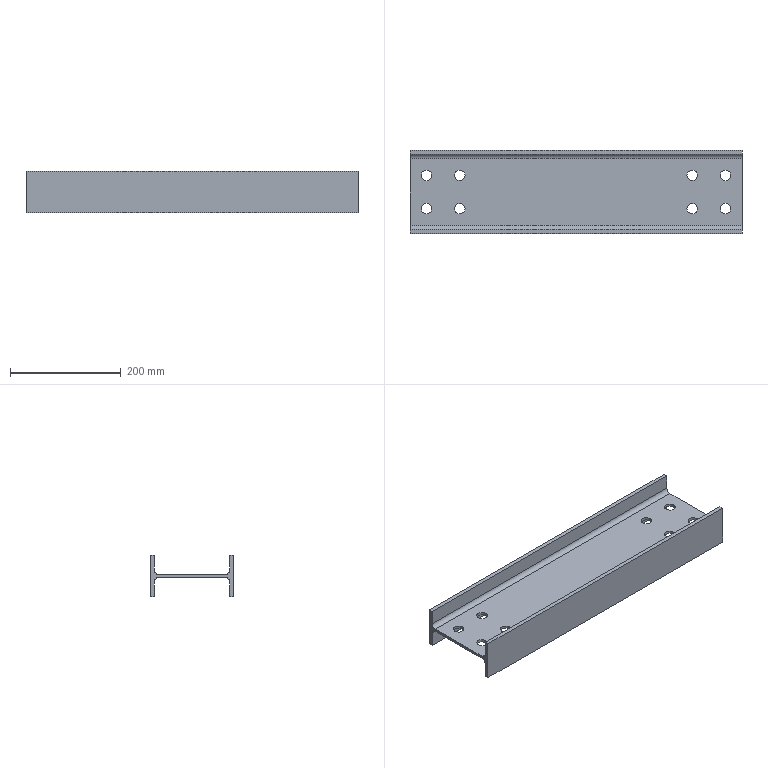Part | STEP file | 计量辅梁8主体_Default<As Machined> | 1 solid | 34 faces | box 600 x 150 x 75 mm | volume 1059622 mm3 | cylinder 20 | plane 14 | commonest cylinder face diameters 19 x16 16 x4